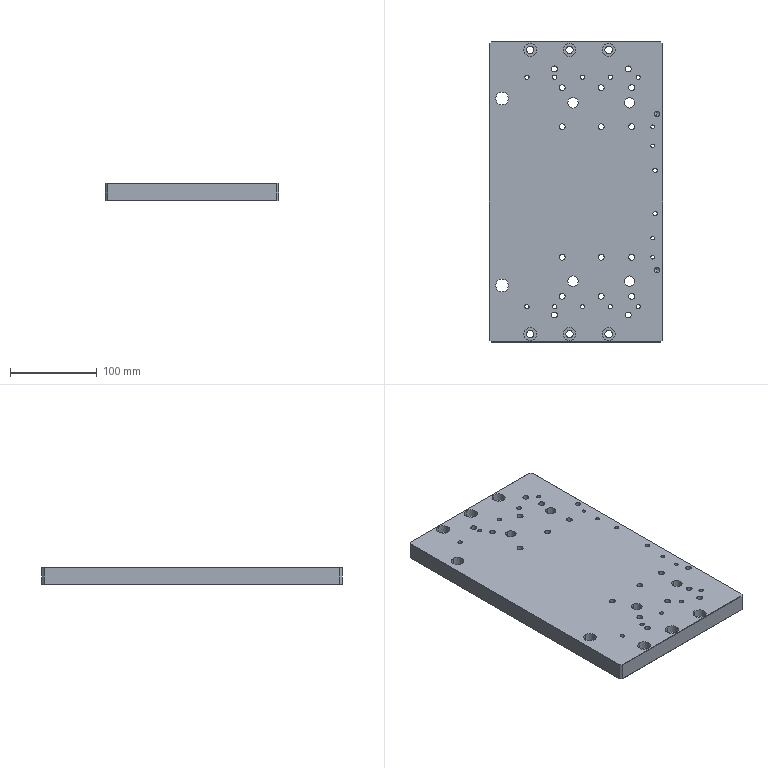NC program | NX | posted with a generic post | part box 200 x 346 x 20 mm
Whole program:
N10 G17 G21 G94 G90
(DRILLING_COPY , TOOL : 8.4ZT)
N12 T16 M6
N14 G54
N16 G17 G0 G90 X-163.5 Y-37.5 S1500 M3
N18 G43 Z30. H16
N20 G94 G83 G98 Z-23.524 F200. Q2. R3.
N22 Y7.5
N24 Y52.5
N26 X163.5
N28 Y7.5
N30 Y-37.5
N32 G80
N34 G0 X163.5 Y-37.5 Z30.
N36 M5
(DRILLING_COPY_COPY , TOOL : 6.8ZT)
N38 T10 M6
N40 G54
N42 G17 G0 G90 X141.5 Y25. S1500 M3
N44 G43 Z30. H10
N46 G94 G83 G98 Z-23.043 F200. Q2. R3.
N48 X120. Y16.
N50 Y-29.
N52 X141.5 Y-60.
N54 X120. Y-64.
N56 X75.
N58 Y-29.
N60 Y16.
N62 X-75.
N64 Y-29.
N66 Y-64.
N68 X-120.
N70 X-141.5 Y-60.
N72 X-120. Y-29.
N74 Y16.
N76 X-141.5 Y25.
N78 G80
N80 G0 X-141.5 Y25. Z30.
N82 M5
(DRILLING_COPY_COPY_COPY , TOOL : 5.0ZT)
N84 T05 M6
N86 G54
N88 G17 G0 G90 X-132. Y56.5 S1500 M3
N90 G43 Z30. H5
N92 G94 G83 G98 Z-22.502 F200. Q2. R3.
N94 Y24.5
N96 Y-7.5
N98 Y-39.5
N100 Y-71.5
N102 X-25. Y-91.
N104 X25.
N106 X132. Y-71.5
N108 Y-39.5
N110 Y-7.5
N112 Y24.5
N114 Y56.5
N116 G80
N118 G0 X132. Y56.5 Z30.
(DRILLING_COPY_COPY_COPY_COPY , TOOL : 5.0ZT)
N120 X-90. Y-93.
N122 G83 Z-16.502 F200. Q2. R3.
N124 X90.
N126 G80
N128 G0 X90. Y-93. Z30.
N130 M5
(DRILLING_COPY_COPY_COPY_COPY_COPY , TOOL : 4.2ZT)
N132 T04 M6
N134 G54
N136 G17 G0 G90 X-75. Y-88. S2122 M3
N138 G43 Z30. H4
N140 G94 G83 G98 Z-22.762 F200. Q2. R3.
N142 X-53.
N144 X53.
N146 X75.
N148 G80
N150 G0 X75. Y-88. Z30.
N152 M5
(DRILLING_COPY_COPY_1 , TOOL : 12.0ZT)
N154 T17 M6
N156 G54
N158 G17 G0 G90 X-102.5 Y3.5 S1500 M3
N160 G43 Z30. H17
N162 G94 G83 G98 Z-24.605 F200. Q2. R3.
N164 Y-61.5
N166 X102.5
N168 Y3.5
N170 G80
N172 G0 X102.5 Y3.5 Z30.
N174 M5
(DRILLING_COPY_COPY_1_COPY , TOOL : 14.5ZT)
N176 T18 M6
N178 G54
N180 G17 G0 G90 X-107.5 Y85. S1500 M3
N182 G43 Z30. H18
N184 G94 G83 G98 Z-25.356 F200. Q2. R3.
N186 X107.5
N188 G80
N190 G0 X107.5 Y85. Z30.
N192 M5
(HOLE_MILLING_COPY , TOOL : D4)
N194 T11 M6
N196 G54
N198 G17 G0 G90 X-90. Y-93. S5000 M3
N200 G43 Z30. H11
N202 Z0.5
N204 G94 G3 X-90.45 Y-93.45 R0.45 F1800.
N206 X-90. Y-93.9 R0.45
N208 X-90. Y-93.9 Z0.35 I0. J0.9
N210 X-90. Y-93.9 Z0.2 I0. J0.9
N212 X-90. Y-93.9 Z0.05 I0. J0.9
N214 X-90. Y-93.9 Z-0.1 I0. J0.9
N216 X-90. Y-93.9 Z-0.25 I0. J0.9
N218 X-90. Y-93.9 Z-0.4 I0. J0.9
N220 X-90. Y-93.9 Z-0.55 I0. J0.9
N222 X-90. Y-93.9 Z-0.7 I0. J0.9
N224 X-90. Y-93.9 Z-0.85 I0. J0.9
N226 X-90. Y-93.9 Z-1. I0. J0.9
N228 X-90. Y-93.9 Z-1.15 I0. J0.9
N230 X-90. Y-93.9 Z-1.3 I0. J0.9
N232 X-90. Y-93.9 Z-1.45 I0. J0.9
N234 X-90. Y-93.9 Z-1.6 I0. J0.9
N236 X-90. Y-93.9 Z-1.75 I0. J0.9
N238 X-90. Y-93.9 Z-1.9 I0. J0.9
N240 X-90. Y-93.9 Z-2.05 I0. J0.9
N242 X-90. Y-93.9 Z-2.2 I0. J0.9
N244 X-90. Y-93.9 Z-2.35 I0. J0.9
N246 X-90. Y-93.9 Z-2.5 I0. J0.9
N248 X-90. Y-93.9 Z-2.65 I0. J0.9
N250 X-90. Y-93.9 Z-2.8 I0. J0.9
N252 X-90. Y-93.9 Z-2.95 I0. J0.9
N254 X-90. Y-93.9 Z-3.1 I0. J0.9
N256 X-90. Y-93.9 Z-3.25 I0. J0.9
N258 X-90. Y-93.9 Z-3.4 I0. J0.9
N260 X-90. Y-93.9 Z-3.55 I0. J0.9
N262 X-90. Y-93.9 Z-3.7 I0. J0.9
N264 X-90. Y-93.9 Z-3.85 I0. J0.9
N266 X-90. Y-93.9 Z-4. I0. J0.9
N268 X-90. Y-93.9 Z-4.15 I0. J0.9
N270 X-90. Y-93.9 Z-4.3 I0. J0.9
N272 X-90. Y-93.9 Z-4.45 I0. J0.9
N274 X-90. Y-93.9 Z-4.6 I0. J0.9
N276 X-90. Y-93.9 Z-4.75 I0. J0.9
N278 X-90. Y-93.9 Z-4.9 I0. J0.9
N280 X-90. Y-93.9 Z-5.05 I0. J0.9
N282 X-90. Y-93.9 Z-5.2 I0. J0.9
N284 X-90. Y-93.9 Z-5.35 I0. J0.9
N286 X-90. Y-93.9 Z-5.5 I0. J0.9
N288 X-90. Y-93.9 Z-5.65 I0. J0.9
N290 X-90. Y-93.9 Z-5.8 I0. J0.9
N292 X-90. Y-93.9 Z-5.95 I0. J0.9
N294 X-90. Y-93.9 Z-6.1 I0. J0.9
N296 X-90. Y-93.9 Z-6.25 I0. J0.9
N298 X-90. Y-93.9 Z-6.4 I0. J0.9
N300 X-90. Y-93.9 Z-6.55 I0. J0.9
N302 X-90. Y-93.9 Z-6.7 I0. J0.9
N304 X-90. Y-93.9 Z-6.85 I0. J0.9
N306 X-90. Y-93.9 Z-7. I0. J0.9
N308 X-90. Y-93.9 Z-7.15 I0. J0.9
N310 X-90. Y-93.9 Z-7.3 I0. J0.9
N312 X-90. Y-93.9 Z-7.45 I0. J0.9
N314 X-90. Y-93.9 Z-7.6 I0. J0.9
N316 X-90. Y-93.9 Z-7.75 I0. J0.9
N318 X-90. Y-93.9 Z-7.9 I0. J0.9
N320 X-90. Y-93.9 Z-8.05 I0. J0.9
N322 X-90. Y-93.9 Z-8.2 I0. J0.9
N324 X-90. Y-93.9 Z-8.35 I0. J0.9
N326 X-90. Y-93.9 Z-8.5 I0. J0.9
N328 X-90. Y-93.9 Z-8.65 I0. J0.9
N330 X-90. Y-93.9 Z-8.8 I0. J0.9
N332 X-90. Y-93.9 Z-8.95 I0. J0.9
N334 X-90. Y-93.9 Z-9.1 I0. J0.9
N336 X-90. Y-93.9 Z-9.25 I0. J0.9
N338 X-90. Y-93.9 Z-9.4 I0. J0.9
N340 X-90. Y-93.9 Z-9.55 I0. J0.9
N342 X-90. Y-93.9 Z-9.7 I0. J0.9
N344 X-90. Y-93.9 Z-9.85 I0. J0.9
N346 X-90. Y-93.9 Z-10. I0. J0.9
N348 X-90. Y-93.9 Z-10.15 I0. J0.9
N350 X-90. Y-93.9 Z-10.3 I0. J0.9
N352 X-90. Y-93.9 Z-10.45 I0. J0.9
N354 X-90. Y-93.9 Z-10.6 I0. J0.9
N356 X-90. Y-93.9 Z-10.75 I0. J0.9
N358 X-90. Y-93.9 Z-10.9 I0. J0.9
N360 X-90. Y-93.9 Z-11.05 I0. J0.9
N362 X-90. Y-93.9 Z-11.2 I0. J0.9
N364 X-90. Y-93.9 Z-11.35 I0. J0.9
N366 X-90. Y-93.9 Z-11.5 I0. J0.9
N368 X-90. Y-93.9 Z-11.65 I0. J0.9
N370 X-90. Y-93.9 Z-11.8 I0. J0.9
N372 X-90. Y-93.9 Z-11.95 I0. J0.9
N374 X-90. Y-93.9 Z-12.1 I0. J0.9
N376 X-90. Y-93.9 Z-12.25 I0. J0.9
N378 X-90. Y-93.9 Z-12.4 I0. J0.9
N380 X-90. Y-93.9 Z-12.55 I0. J0.9
N382 X-90. Y-93.9 Z-12.7 I0. J0.9
N384 X-90. Y-93.9 Z-12.85 I0. J0.9
N386 X-90. Y-93.9 Z-13. I0. J0.9
N388 X-90. Y-93.9 Z-13.15 I0. J0.9
N390 X-90. Y-93.9 Z-13.3 I0. J0.9
N392 X-90. Y-93.9 Z-13.45 I0. J0.9
N394 X-90. Y-93.9 Z-13.6 I0. J0.9
N396 X-90. Y-93.9 Z-13.75 I0. J0.9
N398 X-90. Y-93.9 Z-13.9 I0. J0.9
N400 X-90. Y-93.9 Z-14.05 I0. J0.9
N402 X-90. Y-93.9 Z-14.2 I0. J0.9
N404 X-90. Y-93.9 Z-14.35 I0. J0.9
N406 X-90. Y-93.9 Z-14.5 I0. J0.9
N408 X-90. Y-93.9 Z-14.65 I0. J0.9
N410 X-90. Y-93.9 Z-14.8 I0. J0.9
N412 X-90. Y-93.9 Z-14.95 I0. J0.9
N414 X-89.221 Y-92.55 Z-15. R0.9
N416 X-90.45 Y-92.221 R0.9
N418 X-89.221 Y-92.55 R-0.9
N420 X-89.835 Y-92.385 R0.45
N422 X-90. Y-93. R0.45
N424 G0 Z30.
N426 X90.
N428 Z0.5
N430 G3 X89.55 Y-93.45 R0.45
N432 X90. Y-93.9 R0.45
N434 X90. Y-93.9 Z0.35 I0. J0.9
N436 X90. Y-93.9 Z0.2 I0. J0.9
N438 X90. Y-93.9 Z0.05 I0. J0.9
N440 X90. Y-93.9 Z-0.1 I0. J0.9
N442 X90. Y-93.9 Z-0.25 I0. J0.9
N444 X90. Y-93.9 Z-0.4 I0. J0.9
N446 X90. Y-93.9 Z-0.55 I0. J0.9
N448 X90. Y-93.9 Z-0.7 I0. J0.9
N450 X90. Y-93.9 Z-0.85 I0. J0.9
N452 X90. Y-93.9 Z-1. I0. J0.9
N454 X90. Y-93.9 Z-1.15 I0. J0.9
N456 X90. Y-93.9 Z-1.3 I0. J0.9
N458 X90. Y-93.9 Z-1.45 I0. J0.9
N460 X90. Y-93.9 Z-1.6 I0. J0.9
N462 X90. Y-93.9 Z-1.75 I0. J0.9
N464 X90. Y-93.9 Z-1.9 I0. J0.9
N466 X90. Y-93.9 Z-2.05 I0. J0.9
N468 X90. Y-93.9 Z-2.2 I0. J0.9
N470 X90. Y-93.9 Z-2.35 I0. J0.9
N472 X90. Y-93.9 Z-2.5 I0. J0.9
N474 X90. Y-93.9 Z-2.65 I0. J0.9
N476 X90. Y-93.9 Z-2.8 I0. J0.9
N478 X90. Y-93.9 Z-2.95 I0. J0.9
N480 X90. Y-93.9 Z-3.1 I0. J0.9
N482 X90. Y-93.9 Z-3.25 I0. J0.9
N484 X90. Y-93.9 Z-3.4 I0. J0.9
N486 X90. Y-93.9 Z-3.55 I0. J0.9
N488 X90. Y-93.9 Z-3.7 I0. J0.9
N490 X90. Y-93.9 Z-3.85 I0. J0.9
N492 X90. Y-93.9 Z-4. I0. J0.9
N494 X90. Y-93.9 Z-4.15 I0. J0.9
N496 X90. Y-93.9 Z-4.3 I0. J0.9
N498 X90. Y-93.9 Z-4.45 I0. J0.9
N500 X90. Y-93.9 Z-4.6 I0. J0.9
N502 X90. Y-93.9 Z-4.75 I0. J0.9
N504 X90. Y-93.9 Z-4.9 I0. J0.9
N506 X90. Y-93.9 Z-5.05 I0. J0.9
N508 X90. Y-93.9 Z-5.2 I0. J0.9
N510 X90. Y-93.9 Z-5.35 I0. J0.9
N512 X90. Y-93.9 Z-5.5 I0. J0.9
N514 X90. Y-93.9 Z-5.65 I0. J0.9
N516 X90. Y-93.9 Z-5.8 I0. J0.9
N518 X90. Y-93.9 Z-5.95 I0. J0.9
N520 X90. Y-93.9 Z-6.1 I0. J0.9
N522 X90. Y-93.9 Z-6.25 I0. J0.9
N524 X90. Y-93.9 Z-6.4 I0. J0.9
N526 X90. Y-93.9 Z-6.55 I0. J0.9
N528 X90. Y-93.9 Z-6.7 I0. J0.9
N530 X90. Y-93.9 Z-6.85 I0. J0.9
N532 X90. Y-93.9 Z-7. I0. J0.9
N534 X90. Y-93.9 Z-7.15 I0. J0.9
N536 X90. Y-93.9 Z-7.3 I0. J0.9
N538 X90. Y-93.9 Z-7.45 I0. J0.9
N540 X90. Y-93.9 Z-7.6 I0. J0.9
N542 X90. Y-93.9 Z-7.75 I0. J0.9
N544 X90. Y-93.9 Z-7.9 I0. J0.9
N546 X90. Y-93.9 Z-8.05 I0. J0.9
N548 X90. Y-93.9 Z-8.2 I0. J0.9
N550 X90. Y-93.9 Z-8.35 I0. J0.9
N552 X90. Y-93.9 Z-8.5 I0. J0.9
N554 X90. Y-93.9 Z-8.65 I0. J0.9
N556 X90. Y-93.9 Z-8.8 I0. J0.9
N558 X90. Y-93.9 Z-8.95 I0. J0.9
N560 X90. Y-93.9 Z-9.1 I0. J0.9
N562 X90. Y-93.9 Z-9.25 I0. J0.9
N564 X90. Y-93.9 Z-9.4 I0. J0.9
N566 X90. Y-93.9 Z-9.55 I0. J0.9
N568 X90. Y-93.9 Z-9.7 I0. J0.9
N570 X90. Y-93.9 Z-9.85 I0. J0.9
N572 X90. Y-93.9 Z-10. I0. J0.9
N574 X90. Y-93.9 Z-10.15 I0. J0.9
N576 X90. Y-93.9 Z-10.3 I0. J0.9
N578 X90. Y-93.9 Z-10.45 I0. J0.9
N580 X90. Y-93.9 Z-10.6 I0. J0.9
N582 X90. Y-93.9 Z-10.75 I0. J0.9
N584 X90. Y-93.9 Z-10.9 I0. J0.9
N586 X90. Y-93.9 Z-11.05 I0. J0.9
N588 X90. Y-93.9 Z-11.2 I0. J0.9
N590 X90. Y-93.9 Z-11.35 I0. J0.9
N592 X90. Y-93.9 Z-11.5 I0. J0.9
N594 X90. Y-93.9 Z-11.65 I0. J0.9
N596 X90. Y-93.9 Z-11.8 I0. J0.9
N598 X90. Y-93.9 Z-11.95 I0. J0.9
N600 X90. Y-93.9 Z-12.1 I0. J0.9
N602 X90. Y-93.9 Z-12.25 I0. J0.9
N604 X90. Y-93.9 Z-12.4 I0. J0.9
N606 X90. Y-93.9 Z-12.55 I0. J0.9
N608 X90. Y-93.9 Z-12.7 I0. J0.9
N610 X90. Y-93.9 Z-12.85 I0. J0.9
N612 X90. Y-93.9 Z-13. I0. J0.9
N614 X90. Y-93.9 Z-13.15 I0. J0.9
N616 X90. Y-93.9 Z-13.3 I0. J0.9
N618 X90. Y-93.9 Z-13.45 I0. J0.9
N620 X90. Y-93.9 Z-13.6 I0. J0.9
N622 X90. Y-93.9 Z-13.75 I0. J0.9
N624 X90. Y-93.9 Z-13.9 I0. J0.9
N626 X90. Y-93.9 Z-14.05 I0. J0.9
N628 X90. Y-93.9 Z-14.2 I0. J0.9
N630 X90. Y-93.9 Z-14.35 I0. J0.9
N632 X90. Y-93.9 Z-14.5 I0. J0.9
N634 X90. Y-93.9 Z-14.65 I0. J0.9
N636 X90. Y-93.9 Z-14.8 I0. J0.9
N638 X90. Y-93.9 Z-14.95 I0. J0.9
N640 X90.779 Y-92.55 Z-15. R0.9
N642 X89.55 Y-92.221 R0.9
N644 X90.779 Y-92.55 R-0.9
N646 X90.165 Y-92.385 R0.45
N648 X90. Y-93. R0.45
N650 G0 Z30.
N652 M5
(刀补11 , TOOL : D4)
N654 M6
N656 G54
N658 G17 G0 G90 X-90. Y-93. S5000 M3
N660 G43 Z30. H11
N662 Z0.5
N664 G41 G94 G1 X-90.1 Y-93.004 F1800. D11
N666 G3 X-90. Y-93.94 R0.473
N668 X-90. Y-93.94 Z0.28 I0. J0.94
N670 X-90. Y-93.94 Z0.06 I0. J0.94
N672 X-90. Y-93.94 Z-0.16 I0. J0.94
N674 X-90. Y-93.94 Z-0.38 I0. J0.94
N676 X-90. Y-93.94 Z-0.6 I0. J0.94
N678 X-90. Y-93.94 Z-0.82 I0. J0.94
N680 X-90. Y-93.94 Z-1.04 I0. J0.94
N682 X-90. Y-93.94 Z-1.26 I0. J0.94
N684 X-90. Y-93.94 Z-1.48 I0. J0.94
N686 X-90. Y-93.94 Z-1.7 I0. J0.94
N688 X-90. Y-93.94 Z-1.92 I0. J0.94
N690 X-90. Y-93.94 Z-2.14 I0. J0.94
N692 X-90. Y-93.94 Z-2.36 I0. J0.94
N694 X-90. Y-93.94 Z-2.58 I0. J0.94
N696 X-90. Y-93.94 Z-2.8 I0. J0.94
N698 X-90. Y-93.94 Z-3.02 I0. J0.94
N700 X-90. Y-93.94 Z-3.24 I0. J0.94
N702 X-90. Y-93.94 Z-3.46 I0. J0.94
N704 X-90. Y-93.94 Z-3.68 I0. J0.94
N706 X-90. Y-93.94 Z-3.9 I0. J0.94
N708 X-90. Y-93.94 Z-4.12 I0. J0.94
N710 X-90. Y-93.94 Z-4.34 I0. J0.94
N712 X-90. Y-93.94 Z-4.56 I0. J0.94
N714 X-90. Y-93.94 Z-4.78 I0. J0.94
N716 X-90. Y-93.94 Z-5. I0. J0.94
N718 X-90. Y-93.94 Z-5.22 I0. J0.94
N720 X-90. Y-93.94 Z-5.44 I0. J0.94
N722 X-90. Y-93.94 Z-5.66 I0. J0.94
N724 X-90. Y-93.94 Z-5.88 I0. J0.94
N726 X-90. Y-93.94 Z-6.1 I0. J0.94
N728 X-90. Y-93.94 Z-6.32 I0. J0.94
N730 X-90. Y-93.94 Z-6.54 I0. J0.94
N732 X-90. Y-93.94 Z-6.76 I0. J0.94
N734 X-90. Y-93.94 Z-6.98 I0. J0.94
N736 X-90. Y-93.94 Z-7.2 I0. J0.94
N738 X-90. Y-93.94 Z-7.42 I0. J0.94
N740 X-90. Y-93.94 Z-7.64 I0. J0.94
N742 X-90. Y-93.94 Z-7.86 I0. J0.94
N744 X-90. Y-93.94 Z-8.08 I0. J0.94
N746 X-90. Y-93.94 Z-8.3 I0. J0.94
N748 X-90. Y-93.94 Z-8.52 I0. J0.94
N750 X-90. Y-93.94 Z-8.74 I0. J0.94
N752 X-90. Y-93.94 Z-8.96 I0. J0.94
N754 X-90. Y-93.94 Z-9.18 I0. J0.94
N756 X-90. Y-93.94 Z-9.4 I0. J0.94
N758 X-90. Y-93.94 Z-9.62 I0. J0.94
N760 X-90. Y-93.94 Z-9.84 I0. J0.94
N762 X-90. Y-93.94 Z-10.06 I0. J0.94
N764 X-90. Y-93.94 Z-10.28 I0. J0.94
N766 X-90. Y-93.94 Z-10.5 I0. J0.94
N768 X-90. Y-93.94 Z-10.72 I0. J0.94
N770 X-90. Y-93.94 Z-10.94 I0. J0.94
N772 X-90. Y-93.94 Z-11.16 I0. J0.94
N774 X-90. Y-93.94 Z-11.38 I0. J0.94
N776 X-90. Y-93.94 Z-11.6 I0. J0.94
N778 X-90. Y-93.94 Z-11.82 I0. J0.94
N780 X-90. Y-93.94 Z-12.04 I0. J0.94
N782 X-90. Y-93.94 Z-12.26 I0. J0.94
N784 X-90. Y-93.94 Z-12.48 I0. J0.94
N786 X-90. Y-93.94 Z-12.7 I0. J0.94
N788 X-90. Y-93.94 Z-12.92 I0. J0.94
N790 X-90. Y-93.94 Z-13.14 I0. J0.94
N792 X-90. Y-93.94 Z-13.36 I0. J0.94
N794 X-90. Y-93.94 Z-13.58 I0. J0.94
N796 X-90. Y-93.94 Z-13.8 I0. J0.94
N798 X-90. Y-93.94 Z-14.02 I0. J0.94
N800 X-90. Y-93.94 Z-14.24 I0. J0.94
N802 X-90. Y-93.94 Z-14.46 I0. J0.94
N804 X-90. Y-93.94 Z-14.68 I0. J0.94
N806 X-90. Y-93.94 Z-14.9 I0. J0.94
N808 X-89.735 Y-92.098 Z-15. R0.94
N810 X-90.902 Y-92.735 R0.94
N812 X-89.735 Y-92.098 R-0.94
N814 X-90.095 Y-92.968 R0.473
N816 G40
N818 G1 X-90. Y-93.
N820 G0 Z30.
N822 X90.
N824 Z0.5
N826 G41 G1 X89.9 Y-93.004
N828 G3 X90. Y-93.94 R0.473
N830 X90. Y-93.94 Z0.28 I0. J0.94
N832 X90. Y-93.94 Z0.06 I0. J0.94
N834 X90. Y-93.94 Z-0.16 I0. J0.94
N836 X90. Y-93.94 Z-0.38 I0. J0.94
N838 X90. Y-93.94 Z-0.6 I0. J0.94
N840 X90. Y-93.94 Z-0.82 I0. J0.94
N842 X90. Y-93.94 Z-1.04 I0. J0.94
N844 X90. Y-93.94 Z-1.26 I0. J0.94
N846 X90. Y-93.94 Z-1.48 I0. J0.94
N848 X90. Y-93.94 Z-1.7 I0. J0.94
N850 X90. Y-93.94 Z-1.92 I0. J0.94
N852 X90. Y-93.94 Z-2.14 I0. J0.94
N854 X90. Y-93.94 Z-2.36 I0. J0.94
N856 X90. Y-93.94 Z-2.58 I0. J0.94
N858 X90. Y-93.94 Z-2.8 I0. J0.94
N860 X90. Y-93.94 Z-3.02 I0. J0.94
N862 X90. Y-93.94 Z-3.24 I0. J0.94
N864 X90. Y-93.94 Z-3.46 I0. J0.94
N866 X90. Y-93.94 Z-3.68 I0. J0.94
N868 X90. Y-93.94 Z-3.9 I0. J0.94
N870 X90. Y-93.94 Z-4.12 I0. J0.94
N872 X90. Y-93.94 Z-4.34 I0. J0.94
N874 X90. Y-93.94 Z-4.56 I0. J0.94
N876 X90. Y-93.94 Z-4.78 I0. J0.94
N878 X90. Y-93.94 Z-5. I0. J0.94
N880 X90. Y-93.94 Z-5.22 I0. J0.94
N882 X90. Y-93.94 Z-5.44 I0. J0.94
N884 X90. Y-93.94 Z-5.66 I0. J0.94
N886 X90. Y-93.94 Z-5.88 I0. J0.94
N888 X90. Y-93.94 Z-6.1 I0. J0.94
N890 X90. Y-93.94 Z-6.32 I0. J0.94
N892 X90. Y-93.94 Z-6.54 I0. J0.94
N894 X90. Y-93.94 Z-6.76 I0. J0.94
N896 X90. Y-93.94 Z-6.98 I0. J0.94
N898 X90. Y-93.94 Z-7.2 I0. J0.94
N900 X90. Y-93.94 Z-7.42 I0. J0.94
N902 X90. Y-93.94 Z-7.64 I0. J0.94
N904 X90. Y-93.94 Z-7.86 I0. J0.94
N906 X90. Y-93.94 Z-8.08 I0. J0.94
N908 X90. Y-93.94 Z-8.3 I0. J0.94
N910 X90. Y-93.94 Z-8.52 I0. J0.94
N912 X90. Y-93.94 Z-8.74 I0. J0.94
N914 X90. Y-93.94 Z-8.96 I0. J0.94
N916 X90. Y-93.94 Z-9.18 I0. J0.94
N918 X90. Y-93.94 Z-9.4 I0. J0.94
N920 X90. Y-93.94 Z-9.62 I0. J0.94
N922 X90. Y-93.94 Z-9.84 I0. J0.94
N924 X90. Y-93.94 Z-10.06 I0. J0.94
N926 X90. Y-93.94 Z-10.28 I0. J0.94
N928 X90. Y-93.94 Z-10.5 I0. J0.94
N930 X90. Y-93.94 Z-10.72 I0. J0.94
N932 X90. Y-93.94 Z-10.94 I0. J0.94
N934 X90. Y-93.94 Z-11.16 I0. J0.94
N936 X90. Y-93.94 Z-11.38 I0. J0.94
N938 X90. Y-93.94 Z-11.6 I0. J0.94
N940 X90. Y-93.94 Z-11.82 I0. J0.94
N942 X90. Y-93.94 Z-12.04 I0. J0.94
N944 X90. Y-93.94 Z-12.26 I0. J0.94
N946 X90. Y-93.94 Z-12.48 I0. J0.94
N948 X90. Y-93.94 Z-12.7 I0. J0.94
N950 X90. Y-93.94 Z-12.92 I0. J0.94
N952 X90. Y-93.94 Z-13.14 I0. J0.94
N954 X90. Y-93.94 Z-13.36 I0. J0.94
N956 X90. Y-93.94 Z-13.58 I0. J0.94
N958 X90. Y-93.94 Z-13.8 I0. J0.94
N960 X90. Y-93.94 Z-14.02 I0. J0.94
N962 X90. Y-93.94 Z-14.24 I0. J0.94
N964 X90. Y-93.94 Z-14.46 I0. J0.94
N966 X90. Y-93.94 Z-14.68 I0. J0.94
N968 X90. Y-93.94 Z-14.9 I0. J0.94
N970 X90.265 Y-92.098 Z-15. R0.94
N972 X89.098 Y-92.735 R0.94
N974 X90.265 Y-92.098 R-0.94
N976 X89.905 Y-92.968 R0.473
N978 G40
N980 G1 X90. Y-93.
N982 G0 Z30.
N984 M5
(刀补9 , TOOL : D10M16铣牙刀)
N986 T09 M6
N988 G54
N990 G17 G0 G90 X-107.5 Y85. S2500 M3
N992 G43 Z30. H9
N994 Z1.14
N996 G42 G94 G1 X-109.247 Y85.097 F500. D9
N998 G2 X-109.773 Y86.313 Z1. R0.825
N1000 X-109.773 Y86.313 Z-0.5 I2.273 J-1.312
N1002 X-109.773 Y86.313 Z-2. I2.273 J-1.312
N1004 X-109.773 Y86.313 Z-3.5 I2.273 J-1.312
N1006 X-109.773 Y86.313 Z-5. I2.273 J-1.312
N1008 X-109.773 Y86.313 Z-6.5 I2.273 J-1.312
N1010 X-109.773 Y86.313 Z-8. I2.273 J-1.312
N1012 X-109.773 Y86.313 Z-9.5 I2.273 J-1.312
N1014 X-109.773 Y86.313 Z-11. I2.273 J-1.312
N1016 X-109.773 Y86.313 Z-12.5 I2.273 J-1.312
N1018 X-109.773 Y86.313 Z-14. I2.273 J-1.312
N1020 X-109.773 Y86.313 Z-15.5 I2.273 J-1.312
N1022 X-109.773 Y86.313 Z-17. I2.273 J-1.312
N1024 X-109.773 Y86.313 Z-18.5 I2.273 J-1.312
N1026 X-109.773 Y86.313 Z-20. I2.273 J-1.312
N1028 X-108.458 Y86.465 Z-20.14 R0.825
N1030 G40
N1032 G1 X-107.5 Y85.
N1034 G0 Z1.176
N1036 G42 G1 X-109.244 Y84.853
N1038 G2 X-110.098 Y86.5 Z1. R1.101
N1040 X-110.098 Y86.5 Z-0.5 I2.598 J-1.5
N1042 X-110.098 Y86.5 Z-2. I2.598 J-1.5
N1044 X-110.098 Y86.5 Z-3.5 I2.598 J-1.5
N1046 X-110.098 Y86.5 Z-5. I2.598 J-1.5
N1048 X-110.098 Y86.5 Z-6.5 I2.598 J-1.5
N1050 X-110.098 Y86.5 Z-8. I2.598 J-1.5
N1052 X-110.098 Y86.5 Z-9.5 I2.598 J-1.5
N1054 X-110.098 Y86.5 Z-11. I2.598 J-1.5
N1056 X-110.098 Y86.5 Z-12.5 I2.598 J-1.5
N1058 X-110.098 Y86.5 Z-14. I2.598 J-1.5
N1060 X-110.098 Y86.5 Z-15.5 I2.598 J-1.5
N1062 X-110.098 Y86.5 Z-17. I2.598 J-1.5
N1064 X-110.098 Y86.5 Z-18.5 I2.598 J-1.5
N1066 X-110.098 Y86.5 Z-20. I2.598 J-1.5
N1068 X-108.244 Y86.584 Z-20.176 R1.101
N1070 G40
N1072 G1 X-107.5 Y85.
N1074 G0 Z30.
N1076 X107.5
N1078 Z1.14
N1080 G42 G1 X105.753 Y85.097
N1082 G2 X105.227 Y86.313 Z1. R0.825
N1084 X105.227 Y86.313 Z-0.5 I2.273 J-1.312
N1086 X105.227 Y86.313 Z-2. I2.273 J-1.312
N1088 X105.227 Y86.313 Z-3.5 I2.273 J-1.312
N1090 X105.227 Y86.313 Z-5. I2.273 J-1.312
N1092 X105.227 Y86.313 Z-6.5 I2.273 J-1.312
N1094 X105.227 Y86.313 Z-8. I2.273 J-1.312
N1096 X105.227 Y86.313 Z-9.5 I2.273 J-1.312
N1098 X105.227 Y86.313 Z-11. I2.273 J-1.312
N1100 X105.227 Y86.313 Z-12.5 I2.273 J-1.312
N1102 X105.227 Y86.313 Z-14. I2.273 J-1.312
N1104 X105.227 Y86.313 Z-15.5 I2.273 J-1.312
N1106 X105.227 Y86.313 Z-17. I2.273 J-1.312
N1108 X105.227 Y86.313 Z-18.5 I2.273 J-1.312
N1110 X105.227 Y86.313 Z-20. I2.273 J-1.312
N1112 X106.542 Y86.465 Z-20.14 R0.825
N1114 G40
N1116 G1 X107.5 Y85.
N1118 G0 Z1.176
N1120 G42 G1 X105.756 Y84.853
N1122 G2 X104.902 Y86.5 Z1. R1.101
N1124 X104.902 Y86.5 Z-0.5 I2.598 J-1.5
N1126 X104.902 Y86.5 Z-2. I2.598 J-1.5
N1128 X104.902 Y86.5 Z-3.5 I2.598 J-1.5
N1130 X104.902 Y86.5 Z-5. I2.598 J-1.5
N1132 X104.902 Y86.5 Z-6.5 I2.598 J-1.5
N1134 X104.902 Y86.5 Z-8. I2.598 J-1.5
N1136 X104.902 Y86.5 Z-9.5 I2.598 J-1.5
N1138 X104.902 Y86.5 Z-11. I2.598 J-1.5
N1140 X104.902 Y86.5 Z-12.5 I2.598 J-1.5
N1142 X104.902 Y86.5 Z-14. I2.598 J-1.5
N1144 X104.902 Y86.5 Z-15.5 I2.598 J-1.5
N1146 X104.902 Y86.5 Z-17. I2.598 J-1.5
N1148 X104.902 Y86.5 Z-18.5 I2.598 J-1.5
N1150 X104.902 Y86.5 Z-20. I2.598 J-1.5
N1152 X106.756 Y86.584 Z-20.176 R1.101
N1154 G40
N1156 G1 X107.5 Y85.
N1158 G0 Z30.
N1160 M5
N1162 M2